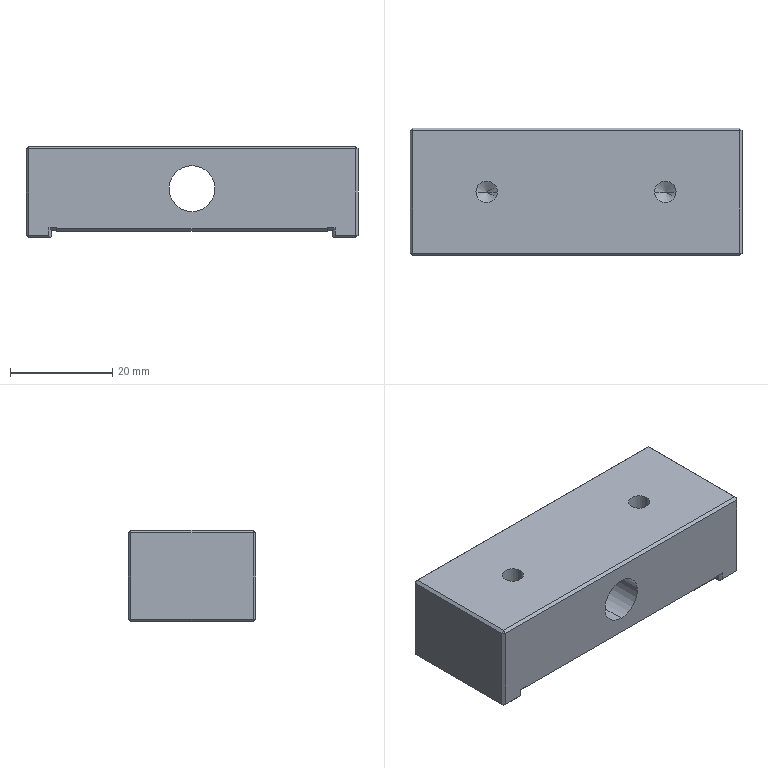Part | SolidWorks | features Chamfer 4, HoleWzd 3, Extrusion 1, ICE 1 | 1 solid | 71 faces | box 65 x 25 x 18 mm | volume 24148 mm3 | plane 49 | cylinder 12 | cone 10 | commonest cylinder face diameters 4.2 x8 9 x2 15 x2